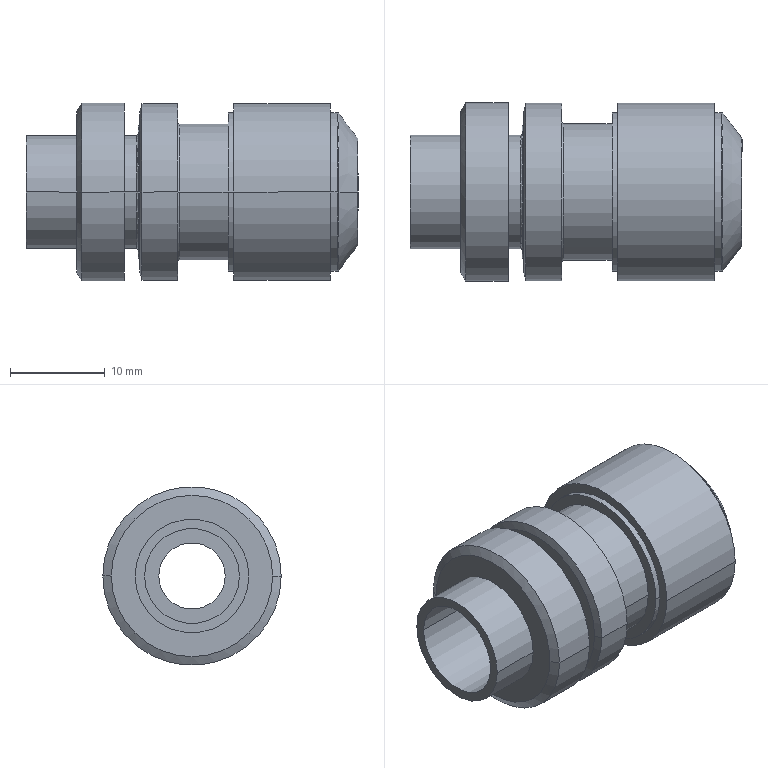Part | STEP file | AG12-6.5 | 1 solid | 47 faces | box 35 x 18.8 x 18.8 mm | volume 5027 mm3 | cylinder 22 | plane 11 | torus 8 | cone 6 | commonest cylinder face diameters 12 x4 16.7 x4 7 x2 10 x2 14 x2 14.4 x2
STEP:
#1=CARTESIAN_POINT('',(35.,3.5,0.));
#2=VERTEX_POINT('',#1);
#3=CARTESIAN_POINT('',(35.,-3.5,0.));
#4=VERTEX_POINT('',#3);
#5=CARTESIAN_POINT('',(35.,0.,0.));
#6=DIRECTION('',(-1.,0.,0.));
#7=DIRECTION('',(0.,1.,0.));
#8=AXIS2_PLACEMENT_3D('',#5,#6,#7);
#9=CIRCLE('',#8,3.5);
#10=EDGE_CURVE('',#2,#4,#9,.T.);
#11=ORIENTED_EDGE('',*,*,#10,.F.);
#12=CARTESIAN_POINT('',(30.,3.5,0.));
#13=VERTEX_POINT('',#12);
#14=CARTESIAN_POINT('',(35.001,3.5,0.));
#15=DIRECTION('',(-1.,0.,0.));
#16=VECTOR('',#15,1000.);
#17=LINE('',#14,#16);
#18=EDGE_CURVE('',#2,#13,#17,.T.);
#19=ORIENTED_EDGE('',*,*,#18,.T.);
#20=CARTESIAN_POINT('',(30.,-3.5,0.));
#21=VERTEX_POINT('',#20);
#22=CARTESIAN_POINT('',(30.,0.,0.));
#23=DIRECTION('',(-1.,0.,0.));
#24=DIRECTION('',(0.,-1.,0.));
#25=AXIS2_PLACEMENT_3D('',#22,#23,#24);
#26=CIRCLE('',#25,3.5);
#27=EDGE_CURVE('',#13,#21,#26,.T.);
#28=ORIENTED_EDGE('',*,*,#27,.T.);
#29=CARTESIAN_POINT('',(35.001,-3.5,0.));
#30=DIRECTION('',(-1.,0.,0.));
#31=VECTOR('',#30,1000.);
#32=LINE('',#29,#31);
#33=EDGE_CURVE('',#4,#21,#32,.T.);
#34=ORIENTED_EDGE('',*,*,#33,.F.);
#35=EDGE_LOOP('',(#11,#19,#28,#34));
#36=FACE_OUTER_BOUND('',#35,.T.);
#37=CARTESIAN_POINT('',(35.001,0.,0.));
#38=DIRECTION('',(-1.,0.,0.));
#39=DIRECTION('',(0.,-1.,0.));
#40=AXIS2_PLACEMENT_3D('',#37,#38,#39);
#41=CYLINDRICAL_SURFACE('',#40,3.5);
#42=ADVANCED_FACE('',(#36),#41,.F.);
#43=CARTESIAN_POINT('',(30.,5.,0.));
#44=VERTEX_POINT('',#43);
#45=CARTESIAN_POINT('',(30.,-5.,0.));
#46=VERTEX_POINT('',#45);
#47=CARTESIAN_POINT('',(30.,0.,0.));
#48=DIRECTION('',(-1.,0.,0.));
#49=DIRECTION('',(0.,-1.,0.));
#50=AXIS2_PLACEMENT_3D('',#47,#48,#49);
#51=CIRCLE('',#50,5.);
#52=EDGE_CURVE('',#44,#46,#51,.T.);
#53=ORIENTED_EDGE('',*,*,#52,.F.);
#54=CARTESIAN_POINT('',(0.,5.,0.));
#55=VERTEX_POINT('',#54);
#56=CARTESIAN_POINT('',(30.,5.,0.));
#57=DIRECTION('',(-1.,0.,0.));
#58=VECTOR('',#57,1000.);
#59=LINE('',#56,#58);
#60=EDGE_CURVE('',#44,#55,#59,.T.);
#61=ORIENTED_EDGE('',*,*,#60,.T.);
#62=CARTESIAN_POINT('',(0.,-5.,0.));
#63=VERTEX_POINT('',#62);
#64=CARTESIAN_POINT('',(0.,0.,0.));
#65=DIRECTION('',(-1.,0.,0.));
#66=DIRECTION('',(0.,-1.,0.));
#67=AXIS2_PLACEMENT_3D('',#64,#65,#66);
#68=CIRCLE('',#67,5.);
#69=EDGE_CURVE('',#55,#63,#68,.T.);
#70=ORIENTED_EDGE('',*,*,#69,.T.);
#71=CARTESIAN_POINT('',(30.,-5.,0.));
#72=DIRECTION('',(-1.,0.,0.));
#73=VECTOR('',#72,1000.);
#74=LINE('',#71,#73);
#75=EDGE_CURVE('',#46,#63,#74,.T.);
#76=ORIENTED_EDGE('',*,*,#75,.F.);
#77=EDGE_LOOP('',(#53,#61,#70,#76));
#78=FACE_OUTER_BOUND('',#77,.T.);
#79=CARTESIAN_POINT('',(30.,0.,0.));
#80=DIRECTION('',(-1.,0.,0.));
#81=DIRECTION('',(0.,-1.,0.));
#82=AXIS2_PLACEMENT_3D('',#79,#80,#81);
#83=CYLINDRICAL_SURFACE('',#82,5.);
#84=ADVANCED_FACE('',(#78),#83,.F.);
#85=CARTESIAN_POINT('',(12.,-7.,0.));
#86=VERTEX_POINT('',#85);
#87=CARTESIAN_POINT('',(12.,7.,0.));
#88=VERTEX_POINT('',#87);
#89=CARTESIAN_POINT('',(12.,0.,0.));
#90=DIRECTION('',(-1.,0.,0.));
#91=DIRECTION('',(0.,-1.,0.));
#92=AXIS2_PLACEMENT_3D('',#89,#90,#91);
#93=CIRCLE('',#92,7.);
#94=EDGE_CURVE('',#86,#88,#93,.T.);
#95=ORIENTED_EDGE('',*,*,#94,.T.);
#96=CARTESIAN_POINT('',(11.85,7.,0.));
#97=VERTEX_POINT('',#96);
#98=CARTESIAN_POINT('',(0.,7.,0.));
#99=DIRECTION('',(-1.,0.,0.));
#100=VECTOR('',#99,1000.);
#101=LINE('',#98,#100);
#102=EDGE_CURVE('',#88,#97,#101,.T.);
#103=ORIENTED_EDGE('',*,*,#102,.T.);
#104=CARTESIAN_POINT('',(11.85,-7.,0.));
#105=VERTEX_POINT('',#104);
#106=CARTESIAN_POINT('',(11.85,0.,0.));
#107=DIRECTION('',(-1.,0.,0.));
#108=DIRECTION('',(0.,-1.,0.));
#109=AXIS2_PLACEMENT_3D('',#106,#107,#108);
#110=CIRCLE('',#109,7.);
#111=EDGE_CURVE('',#105,#97,#110,.T.);
#112=ORIENTED_EDGE('',*,*,#111,.F.);
#113=CARTESIAN_POINT('',(0.,-7.,0.));
#114=DIRECTION('',(-1.,0.,0.));
#115=VECTOR('',#114,1000.);
#116=LINE('',#113,#115);
#117=EDGE_CURVE('',#86,#105,#116,.T.);
#118=ORIENTED_EDGE('',*,*,#117,.F.);
#119=EDGE_LOOP('',(#95,#103,#112,#118));
#120=FACE_OUTER_BOUND('',#119,.T.);
#121=CARTESIAN_POINT('',(0.,0.,0.));
#122=DIRECTION('',(-1.,0.,0.));
#123=DIRECTION('',(0.,-1.,0.));
#124=AXIS2_PLACEMENT_3D('',#121,#122,#123);
#125=CYLINDRICAL_SURFACE('',#124,7.);
#126=ADVANCED_FACE('',(#120),#125,.T.);
#127=CARTESIAN_POINT('',(12.,-8.5,0.));
#128=VERTEX_POINT('',#127);
#129=CARTESIAN_POINT('',(12.,8.5,0.));
#130=VERTEX_POINT('',#129);
#131=CARTESIAN_POINT('',(12.,0.,0.));
#132=DIRECTION('',(-1.,0.,0.));
#133=DIRECTION('',(0.,-1.,0.));
#134=AXIS2_PLACEMENT_3D('',#131,#132,#133);
#135=CIRCLE('',#134,8.5);
#136=EDGE_CURVE('',#128,#130,#135,.T.);
#137=ORIENTED_EDGE('',*,*,#136,.F.);
#138=CARTESIAN_POINT('',(12.228,-9.35,0.));
#139=VERTEX_POINT('',#138);
#140=CARTESIAN_POINT('',(12.,-8.5,0.));
#141=DIRECTION('',(0.2588,-0.9659,0.));
#142=VECTOR('',#141,1000.);
#143=LINE('',#140,#142);
#144=EDGE_CURVE('',#128,#139,#143,.T.);
#145=ORIENTED_EDGE('',*,*,#144,.T.);
#146=CARTESIAN_POINT('',(12.228,9.35,0.));
#147=VERTEX_POINT('',#146);
#148=CARTESIAN_POINT('',(12.228,0.,0.));
#149=DIRECTION('',(-1.,0.,0.));
#150=DIRECTION('',(0.,-1.,0.));
#151=AXIS2_PLACEMENT_3D('',#148,#149,#150);
#152=CIRCLE('',#151,9.35);
#153=EDGE_CURVE('',#139,#147,#152,.T.);
#154=ORIENTED_EDGE('',*,*,#153,.T.);
#155=CARTESIAN_POINT('',(12.,8.5,0.));
#156=DIRECTION('',(0.2588,0.9659,0.));
#157=VECTOR('',#156,1000.);
#158=LINE('',#155,#157);
#159=EDGE_CURVE('',#130,#147,#158,.T.);
#160=ORIENTED_EDGE('',*,*,#159,.F.);
#161=EDGE_LOOP('',(#137,#145,#154,#160));
#162=FACE_OUTER_BOUND('',#161,.T.);
#163=CARTESIAN_POINT('',(12.,0.,0.));
#164=DIRECTION('',(1.,0.,0.));
#165=DIRECTION('',(0.,1.,0.));
#166=AXIS2_PLACEMENT_3D('',#163,#164,#165);
#167=CONICAL_SURFACE('',#166,8.5,1.309);
#168=ADVANCED_FACE('',(#162),#167,.T.);
#169=CARTESIAN_POINT('',(16.,-9.35,0.));
#170=VERTEX_POINT('',#169);
#171=CARTESIAN_POINT('',(16.,9.35,0.));
#172=VERTEX_POINT('',#171);
#173=CARTESIAN_POINT('',(16.,0.,0.));
#174=DIRECTION('',(-1.,0.,0.));
#175=DIRECTION('',(0.,-1.,0.));
#176=AXIS2_PLACEMENT_3D('',#173,#174,#175);
#177=CIRCLE('',#176,9.35);
#178=EDGE_CURVE('',#170,#172,#177,.T.);
#179=ORIENTED_EDGE('',*,*,#178,.T.);
#180=CARTESIAN_POINT('',(0.,9.35,0.));
#181=DIRECTION('',(-1.,0.,0.));
#182=VECTOR('',#181,1000.);
#183=LINE('',#180,#182);
#184=EDGE_CURVE('',#172,#147,#183,.T.);
#185=ORIENTED_EDGE('',*,*,#184,.T.);
#186=ORIENTED_EDGE('',*,*,#153,.F.);
#187=CARTESIAN_POINT('',(0.,-9.35,0.));
#188=DIRECTION('',(-1.,0.,0.));
#189=VECTOR('',#188,1000.);
#190=LINE('',#187,#189);
#191=EDGE_CURVE('',#170,#139,#190,.T.);
#192=ORIENTED_EDGE('',*,*,#191,.F.);
#193=EDGE_LOOP('',(#179,#185,#186,#192));
#194=FACE_OUTER_BOUND('',#193,.T.);
#195=CARTESIAN_POINT('',(0.,0.,0.));
#196=DIRECTION('',(-1.,0.,0.));
#197=DIRECTION('',(0.,-1.,0.));
#198=AXIS2_PLACEMENT_3D('',#195,#196,#197);
#199=CYLINDRICAL_SURFACE('',#198,9.35);
#200=ADVANCED_FACE('',(#194),#199,.T.);
#201=CARTESIAN_POINT('',(16.,7.4,0.));
#202=VERTEX_POINT('',#201);
#203=CARTESIAN_POINT('',(16.,-7.4,0.));
#204=VERTEX_POINT('',#203);
#205=CARTESIAN_POINT('',(16.,0.,0.));
#206=DIRECTION('',(-1.,0.,0.));
#207=DIRECTION('',(0.,-1.,0.));
#208=AXIS2_PLACEMENT_3D('',#205,#206,#207);
#209=CIRCLE('',#208,7.4);
#210=EDGE_CURVE('',#202,#204,#209,.T.);
#211=ORIENTED_EDGE('',*,*,#210,.F.);
#212=CARTESIAN_POINT('',(16.2,7.2,0.));
#213=VERTEX_POINT('',#212);
#214=CARTESIAN_POINT('',(16.2,7.4,0.));
#215=DIRECTION('',(0.,0.,1.));
#216=DIRECTION('',(0.,-1.,0.));
#217=AXIS2_PLACEMENT_3D('',#214,#215,#216);
#218=CIRCLE('',#217,0.2);
#219=EDGE_CURVE('',#202,#213,#218,.T.);
#220=ORIENTED_EDGE('',*,*,#219,.T.);
#221=CARTESIAN_POINT('',(16.2,-7.2,0.));
#222=VERTEX_POINT('',#221);
#223=CARTESIAN_POINT('',(16.2,0.,0.));
#224=DIRECTION('',(-1.,0.,0.));
#225=DIRECTION('',(0.,-1.,0.));
#226=AXIS2_PLACEMENT_3D('',#223,#224,#225);
#227=CIRCLE('',#226,7.2);
#228=EDGE_CURVE('',#213,#222,#227,.T.);
#229=ORIENTED_EDGE('',*,*,#228,.T.);
#230=CARTESIAN_POINT('',(16.2,-7.4,0.));
#231=DIRECTION('',(0.,0.,-1.));
#232=DIRECTION('',(0.,1.,0.));
#233=AXIS2_PLACEMENT_3D('',#230,#231,#232);
#234=CIRCLE('',#233,0.2);
#235=EDGE_CURVE('',#204,#222,#234,.T.);
#236=ORIENTED_EDGE('',*,*,#235,.F.);
#237=EDGE_LOOP('',(#211,#220,#229,#236));
#238=FACE_OUTER_BOUND('',#237,.T.);
#239=CARTESIAN_POINT('',(16.2,0.,0.));
#240=DIRECTION('',(-1.,0.,0.));
#241=DIRECTION('',(0.,-1.,0.));
#242=AXIS2_PLACEMENT_3D('',#239,#240,#241);
#243=TOROIDAL_SURFACE('',#242,7.4,0.2);
#244=ADVANCED_FACE('',(#238),#243,.F.);
#245=CARTESIAN_POINT('',(21.3,-7.2,0.));
#246=VERTEX_POINT('',#245);
#247=CARTESIAN_POINT('',(21.3,7.2,0.));
#248=VERTEX_POINT('',#247);
#249=CARTESIAN_POINT('',(21.3,0.,0.));
#250=DIRECTION('',(-1.,0.,0.));
#251=DIRECTION('',(0.,-1.,0.));
#252=AXIS2_PLACEMENT_3D('',#249,#250,#251);
#253=CIRCLE('',#252,7.2);
#254=EDGE_CURVE('',#246,#248,#253,.T.);
#255=ORIENTED_EDGE('',*,*,#254,.T.);
#256=CARTESIAN_POINT('',(0.,7.2,0.));
#257=DIRECTION('',(-1.,0.,0.));
#258=VECTOR('',#257,1000.);
#259=LINE('',#256,#258);
#260=EDGE_CURVE('',#248,#213,#259,.T.);
#261=ORIENTED_EDGE('',*,*,#260,.T.);
#262=CARTESIAN_POINT('',(16.2,0.,0.));
#263=DIRECTION('',(-1.,0.,0.));
#264=DIRECTION('',(0.,-1.,0.));
#265=AXIS2_PLACEMENT_3D('',#262,#263,#264);
#266=CIRCLE('',#265,7.2);
#267=EDGE_CURVE('',#222,#213,#266,.T.);
#268=ORIENTED_EDGE('',*,*,#267,.F.);
#269=CARTESIAN_POINT('',(0.,-7.2,0.));
#270=DIRECTION('',(-1.,0.,0.));
#271=VECTOR('',#270,1000.);
#272=LINE('',#269,#271);
#273=EDGE_CURVE('',#246,#222,#272,.T.);
#274=ORIENTED_EDGE('',*,*,#273,.F.);
#275=EDGE_LOOP('',(#255,#261,#268,#274));
#276=FACE_OUTER_BOUND('',#275,.T.);
#277=CARTESIAN_POINT('',(0.,0.,0.));
#278=DIRECTION('',(-1.,0.,0.));
#279=DIRECTION('',(0.,-1.,0.));
#280=AXIS2_PLACEMENT_3D('',#277,#278,#279);
#281=CYLINDRICAL_SURFACE('',#280,7.2);
#282=ADVANCED_FACE('',(#276),#281,.T.);
#283=CARTESIAN_POINT('',(21.9,-8.35,0.));
#284=VERTEX_POINT('',#283);
#285=CARTESIAN_POINT('',(21.9,8.35,0.));
#286=VERTEX_POINT('',#285);
#287=CARTESIAN_POINT('',(21.9,0.,0.));
#288=DIRECTION('',(-1.,0.,0.));
#289=DIRECTION('',(0.,-1.,0.));
#290=AXIS2_PLACEMENT_3D('',#287,#288,#289);
#291=CIRCLE('',#290,8.35);
#292=EDGE_CURVE('',#284,#286,#291,.T.);
#293=ORIENTED_EDGE('',*,*,#292,.T.);
#294=CARTESIAN_POINT('',(21.3,8.35,0.));
#295=VERTEX_POINT('',#294);
#296=CARTESIAN_POINT('',(0.,8.35,0.));
#297=DIRECTION('',(-1.,0.,0.));
#298=VECTOR('',#297,1000.);
#299=LINE('',#296,#298);
#300=EDGE_CURVE('',#286,#295,#299,.T.);
#301=ORIENTED_EDGE('',*,*,#300,.T.);
#302=CARTESIAN_POINT('',(21.3,-8.35,0.));
#303=VERTEX_POINT('',#302);
#304=CARTESIAN_POINT('',(21.3,0.,0.));
#305=DIRECTION('',(-1.,0.,0.));
#306=DIRECTION('',(0.,-1.,0.));
#307=AXIS2_PLACEMENT_3D('',#304,#305,#306);
#308=CIRCLE('',#307,8.35);
#309=EDGE_CURVE('',#303,#295,#308,.T.);
#310=ORIENTED_EDGE('',*,*,#309,.F.);
#311=CARTESIAN_POINT('',(0.,-8.35,0.));
#312=DIRECTION('',(-1.,0.,0.));
#313=VECTOR('',#312,1000.);
#314=LINE('',#311,#313);
#315=EDGE_CURVE('',#284,#303,#314,.T.);
#316=ORIENTED_EDGE('',*,*,#315,.F.);
#317=EDGE_LOOP('',(#293,#301,#310,#316));
#318=FACE_OUTER_BOUND('',#317,.T.);
#319=CARTESIAN_POINT('',(0.,0.,0.));
#320=DIRECTION('',(-1.,0.,0.));
#321=DIRECTION('',(0.,-1.,0.));
#322=AXIS2_PLACEMENT_3D('',#319,#320,#321);
#323=CYLINDRICAL_SURFACE('',#322,8.35);
#324=ADVANCED_FACE('',(#318),#323,.T.);
#325=CARTESIAN_POINT('',(32.1,-9.365,0.));
#326=VERTEX_POINT('',#325);
#327=CARTESIAN_POINT('',(32.1,9.365,0.));
#328=VERTEX_POINT('',#327);
#329=CARTESIAN_POINT('',(32.1,0.,0.));
#330=DIRECTION('',(-1.,0.,0.));
#331=DIRECTION('',(0.,-1.,0.));
#332=AXIS2_PLACEMENT_3D('',#329,#330,#331);
#333=CIRCLE('',#332,9.365);
#334=EDGE_CURVE('',#326,#328,#333,.T.);
#335=ORIENTED_EDGE('',*,*,#334,.T.);
#336=CARTESIAN_POINT('',(21.9,9.365,0.));
#337=VERTEX_POINT('',#336);
#338=CARTESIAN_POINT('',(0.,9.365,0.));
#339=DIRECTION('',(-1.,0.,0.));
#340=VECTOR('',#339,1000.);
#341=LINE('',#338,#340);
#342=EDGE_CURVE('',#328,#337,#341,.T.);
#343=ORIENTED_EDGE('',*,*,#342,.T.);
#344=CARTESIAN_POINT('',(21.9,-9.365,0.));
#345=VERTEX_POINT('',#344);
#346=CARTESIAN_POINT('',(21.9,0.,0.));
#347=DIRECTION('',(-1.,0.,0.));
#348=DIRECTION('',(0.,-1.,0.));
#349=AXIS2_PLACEMENT_3D('',#346,#347,#348);
#350=CIRCLE('',#349,9.365);
#351=EDGE_CURVE('',#345,#337,#350,.T.);
#352=ORIENTED_EDGE('',*,*,#351,.F.);
#353=CARTESIAN_POINT('',(0.,-9.365,0.));
#354=DIRECTION('',(-1.,0.,0.));
#355=VECTOR('',#354,1000.);
#356=LINE('',#353,#355);
#357=EDGE_CURVE('',#326,#345,#356,.T.);
#358=ORIENTED_EDGE('',*,*,#357,.F.);
#359=EDGE_LOOP('',(#335,#343,#352,#358));
#360=FACE_OUTER_BOUND('',#359,.T.);
#361=CARTESIAN_POINT('',(0.,0.,0.));
#362=DIRECTION('',(-1.,0.,0.));
#363=DIRECTION('',(0.,-1.,0.));
#364=AXIS2_PLACEMENT_3D('',#361,#362,#363);
#365=CYLINDRICAL_SURFACE('',#364,9.365);
#366=ADVANCED_FACE('',(#360),#365,.T.);
#367=CARTESIAN_POINT('',(32.837,-8.35,0.));
#368=VERTEX_POINT('',#367);
#369=CARTESIAN_POINT('',(32.837,8.35,0.));
#370=VERTEX_POINT('',#369);
#371=CARTESIAN_POINT('',(32.837,0.,0.));
#372=DIRECTION('',(-1.,0.,0.));
#373=DIRECTION('',(0.,-1.,0.));
#374=AXIS2_PLACEMENT_3D('',#371,#372,#373);
#375=CIRCLE('',#374,8.35);
#376=EDGE_CURVE('',#368,#370,#375,.T.);
#377=ORIENTED_EDGE('',*,*,#376,.T.);
#378=CARTESIAN_POINT('',(32.1,8.35,0.));
#379=VERTEX_POINT('',#378);
#380=CARTESIAN_POINT('',(0.,8.35,0.));
#381=DIRECTION('',(-1.,0.,0.));
#382=VECTOR('',#381,1000.);
#383=LINE('',#380,#382);
#384=EDGE_CURVE('',#370,#379,#383,.T.);
#385=ORIENTED_EDGE('',*,*,#384,.T.);
#386=CARTESIAN_POINT('',(32.1,-8.35,0.));
#387=VERTEX_POINT('',#386);
#388=CARTESIAN_POINT('',(32.1,0.,0.));
#389=DIRECTION('',(-1.,0.,0.));
#390=DIRECTION('',(0.,-1.,0.));
#391=AXIS2_PLACEMENT_3D('',#388,#389,#390);
#392=CIRCLE('',#391,8.35);
#393=EDGE_CURVE('',#387,#379,#392,.T.);
#394=ORIENTED_EDGE('',*,*,#393,.F.);
#395=CARTESIAN_POINT('',(0.,-8.35,0.));
#396=DIRECTION('',(-1.,0.,0.));
#397=VECTOR('',#396,1000.);
#398=LINE('',#395,#397);
#399=EDGE_CURVE('',#368,#387,#398,.T.);
#400=ORIENTED_EDGE('',*,*,#399,.F.);
#401=EDGE_LOOP('',(#377,#385,#394,#400));
#402=FACE_OUTER_BOUND('',#401,.T.);
#403=CARTESIAN_POINT('',(0.,0.,0.));
#404=DIRECTION('',(-1.,0.,0.));
#405=DIRECTION('',(0.,-1.,0.));
#406=AXIS2_PLACEMENT_3D('',#403,#404,#405);
#407=CYLINDRICAL_SURFACE('',#406,8.35);
#408=ADVANCED_FACE('',(#402),#407,.T.);
#409=CARTESIAN_POINT('',(32.996,-8.271,0.));
#410=VERTEX_POINT('',#409);
#411=CARTESIAN_POINT('',(32.996,8.271,0.));
#412=VERTEX_POINT('',#411);
#413=CARTESIAN_POINT('',(32.996,0.,0.));
#414=DIRECTION('',(-1.,0.,0.));
#415=DIRECTION('',(0.,-1.,0.));
#416=AXIS2_PLACEMENT_3D('',#413,#414,#415);
#417=CIRCLE('',#416,8.271);
#418=EDGE_CURVE('',#410,#412,#417,.T.);
#419=ORIENTED_EDGE('',*,*,#418,.T.);
#420=CARTESIAN_POINT('',(32.837,8.15,0.));
#421=DIRECTION('',(0.,0.,1.));
#422=DIRECTION('',(0.,-1.,0.));
#423=AXIS2_PLACEMENT_3D('',#420,#421,#422);
#424=CIRCLE('',#423,0.2);
#425=EDGE_CURVE('',#412,#370,#424,.T.);
#426=ORIENTED_EDGE('',*,*,#425,.T.);
#427=ORIENTED_EDGE('',*,*,#376,.F.);
#428=CARTESIAN_POINT('',(32.837,-8.15,0.));
#429=DIRECTION('',(0.,0.,-1.));
#430=DIRECTION('',(0.,1.,0.));
#431=AXIS2_PLACEMENT_3D('',#428,#429,#430);
#432=CIRCLE('',#431,0.2);
#433=EDGE_CURVE('',#410,#368,#432,.T.);
#434=ORIENTED_EDGE('',*,*,#433,.F.);
#435=EDGE_LOOP('',(#419,#426,#427,#434));
#436=FACE_OUTER_BOUND('',#435,.T.);
#437=CARTESIAN_POINT('',(32.837,0.,0.));
#438=DIRECTION('',(-1.,0.,0.));
#439=DIRECTION('',(0.,-1.,0.));
#440=AXIS2_PLACEMENT_3D('',#437,#438,#439);
#441=TOROIDAL_SURFACE('',#440,8.15,0.2);
#442=ADVANCED_FACE('',(#436),#441,.T.);
#443=CARTESIAN_POINT('',(34.959,-5.704,0.));
#444=VERTEX_POINT('',#443);
#445=CARTESIAN_POINT('',(34.959,5.704,0.));
#446=VERTEX_POINT('',#445);
#447=CARTESIAN_POINT('',(34.959,0.,0.));
#448=DIRECTION('',(-1.,0.,0.));
#449=DIRECTION('',(0.,-1.,0.));
#450=AXIS2_PLACEMENT_3D('',#447,#448,#449);
#451=CIRCLE('',#450,5.704);
#452=EDGE_CURVE('',#444,#446,#451,.T.);
#453=ORIENTED_EDGE('',*,*,#452,.T.);
#454=CARTESIAN_POINT('',(34.959,5.704,0.));
#455=DIRECTION('',(-0.6074,0.7944,0.));
#456=VECTOR('',#455,1000.);
#457=LINE('',#454,#456);
#458=EDGE_CURVE('',#446,#412,#457,.T.);
#459=ORIENTED_EDGE('',*,*,#458,.T.);
#460=ORIENTED_EDGE('',*,*,#418,.F.);
#461=CARTESIAN_POINT('',(34.959,-5.704,0.));
#462=DIRECTION('',(-0.6074,-0.7944,0.));
#463=VECTOR('',#462,1000.);
#464=LINE('',#461,#463);
#465=EDGE_CURVE('',#444,#410,#464,.T.);
#466=ORIENTED_EDGE('',*,*,#465,.F.);
#467=EDGE_LOOP('',(#453,#459,#460,#466));
#468=FACE_OUTER_BOUND('',#467,.T.);
#469=CARTESIAN_POINT('',(34.959,0.,0.));
#470=DIRECTION('',(-1.,0.,0.));
#471=DIRECTION('',(0.,-1.,0.));
#472=AXIS2_PLACEMENT_3D('',#469,#470,#471);
#473=CONICAL_SURFACE('',#472,5.704,0.918);
#474=ADVANCED_FACE('',(#468),#473,.T.);
#475=CARTESIAN_POINT('',(35.,-5.582,0.));
#476=VERTEX_POINT('',#475);
#477=CARTESIAN_POINT('',(35.,5.582,0.));
#478=VERTEX_POINT('',#477);
#479=CARTESIAN_POINT('',(35.,0.,0.));
#480=DIRECTION('',(-1.,0.,0.));
#481=DIRECTION('',(0.,-1.,0.));
#482=AXIS2_PLACEMENT_3D('',#479,#480,#481);
#483=CIRCLE('',#482,5.582);
#484=EDGE_CURVE('',#476,#478,#483,.T.);
#485=ORIENTED_EDGE('',*,*,#484,.T.);
#486=CARTESIAN_POINT('',(34.8,5.582,0.));
#487=DIRECTION('',(0.,0.,1.));
#488=DIRECTION('',(0.,-1.,0.));
#489=AXIS2_PLACEMENT_3D('',#486,#487,#488);
#490=CIRCLE('',#489,0.2);
#491=EDGE_CURVE('',#478,#446,#490,.T.);
#492=ORIENTED_EDGE('',*,*,#491,.T.);
#493=ORIENTED_EDGE('',*,*,#452,.F.);
#494=CARTESIAN_POINT('',(34.8,-5.582,0.));
#495=DIRECTION('',(0.,0.,-1.));
#496=DIRECTION('',(0.,1.,0.));
#497=AXIS2_PLACEMENT_3D('',#494,#495,#496);
#498=CIRCLE('',#497,0.2);
#499=EDGE_CURVE('',#476,#444,#498,.T.);
#500=ORIENTED_EDGE('',*,*,#499,.F.);
#501=EDGE_LOOP('',(#485,#492,#493,#500));
#502=FACE_OUTER_BOUND('',#501,.T.);
#503=CARTESIAN_POINT('',(34.8,0.,0.));
#504=DIRECTION('',(-1.,0.,0.));
#505=DIRECTION('',(0.,-1.,0.));
#506=AXIS2_PLACEMENT_3D('',#503,#504,#505);
#507=TOROIDAL_SURFACE('',#506,5.582,0.2);
#508=ADVANCED_FACE('',(#502),#507,.T.);
#509=CARTESIAN_POINT('',(5.35,-6.,0.));
#510=VERTEX_POINT('',#509);
#511=CARTESIAN_POINT('',(5.35,6.,0.));
#512=VERTEX_POINT('',#511);
#513=CARTESIAN_POINT('',(5.35,0.,0.));
#514=DIRECTION('',(-1.,0.,0.));
#515=DIRECTION('',(0.,-1.,0.));
#516=AXIS2_PLACEMENT_3D('',#513,#514,#515);
#517=CIRCLE('',#516,6.);
#518=EDGE_CURVE('',#510,#512,#517,.T.);
#519=ORIENTED_EDGE('',*,*,#518,.T.);
#520=CARTESIAN_POINT('',(0.,6.,0.));
#521=VERTEX_POINT('',#520);
#522=CARTESIAN_POINT('',(0.,6.,0.));
#523=DIRECTION('',(-1.,0.,0.));
#524=VECTOR('',#523,1000.);
#525=LINE('',#522,#524);
#526=EDGE_CURVE('',#512,#521,#525,.T.);
#527=ORIENTED_EDGE('',*,*,#526,.T.);
#528=CARTESIAN_POINT('',(0.,-6.,0.));
#529=VERTEX_POINT('',#528);
#530=CARTESIAN_POINT('',(0.,0.,0.));
#531=DIRECTION('',(-1.,0.,0.));
#532=DIRECTION('',(0.,-1.,0.));
#533=AXIS2_PLACEMENT_3D('',#530,#531,#532);
#534=CIRCLE('',#533,6.);
#535=EDGE_CURVE('',#529,#521,#534,.T.);
#536=ORIENTED_EDGE('',*,*,#535,.F.);
#537=CARTESIAN_POINT('',(0.,-6.,0.));
#538=DIRECTION('',(-1.,0.,0.));
#539=VECTOR('',#538,1000.);
#540=LINE('',#537,#539);
#541=EDGE_CURVE('',#510,#529,#540,.T.);
#542=ORIENTED_EDGE('',*,*,#541,.F.);
#543=EDGE_LOOP('',(#519,#527,#536,#542));
#544=FACE_OUTER_BOUND('',#543,.T.);
#545=CARTESIAN_POINT('',(0.,0.,0.));
#546=DIRECTION('',(-1.,0.,0.));
#547=DIRECTION('',(0.,-1.,0.));
#548=AXIS2_PLACEMENT_3D('',#545,#546,#547);
#549=CYLINDRICAL_SURFACE('',#548,6.);
#550=ADVANCED_FACE('',(#544),#549,.T.);
#551=CARTESIAN_POINT('',(5.35,-8.5,0.));
#552=VERTEX_POINT('',#551);
#553=CARTESIAN_POINT('',(5.35,8.5,0.));
#554=VERTEX_POINT('',#553);
#555=CARTESIAN_POINT('',(5.35,0.,0.));
#556=DIRECTION('',(-1.,0.,0.));
#557=DIRECTION('',(0.,-1.,0.));
#558=AXIS2_PLACEMENT_3D('',#555,#556,#557);
#559=CIRCLE('',#558,8.5);
#560=EDGE_CURVE('',#552,#554,#559,.T.);
#561=ORIENTED_EDGE('',*,*,#560,.F.);
#562=CARTESIAN_POINT('',(5.87,-9.4,0.));
#563=VERTEX_POINT('',#562);
#564=CARTESIAN_POINT('',(5.35,-8.5,0.));
#565=DIRECTION('',(0.5,-0.866,0.));
#566=VECTOR('',#565,1000.);
#567=LINE('',#564,#566);
#568=EDGE_CURVE('',#552,#563,#567,.T.);
#569=ORIENTED_EDGE('',*,*,#568,.T.);
#570=CARTESIAN_POINT('',(5.87,9.4,0.));
#571=VERTEX_POINT('',#570);
#572=CARTESIAN_POINT('',(5.87,0.,0.));
#573=DIRECTION('',(-1.,0.,0.));
#574=DIRECTION('',(0.,-1.,0.));
#575=AXIS2_PLACEMENT_3D('',#572,#573,#574);
#576=CIRCLE('',#575,9.4);
#577=EDGE_CURVE('',#563,#571,#576,.T.);
#578=ORIENTED_EDGE('',*,*,#577,.T.);
#579=CARTESIAN_POINT('',(5.35,8.5,0.));
#580=DIRECTION('',(0.5,0.866,0.));
#581=VECTOR('',#580,1000.);
#582=LINE('',#579,#581);
#583=EDGE_CURVE('',#554,#571,#582,.T.);
#584=ORIENTED_EDGE('',*,*,#583,.F.);
#585=EDGE_LOOP('',(#561,#569,#578,#584));
#586=FACE_OUTER_BOUND('',#585,.T.);
#587=CARTESIAN_POINT('',(5.35,0.,0.));
#588=DIRECTION('',(1.,0.,0.));
#589=DIRECTION('',(0.,1.,0.));
#590=AXIS2_PLACEMENT_3D('',#587,#588,#589);
#591=CONICAL_SURFACE('',#590,8.5,1.047);
#592=ADVANCED_FACE('',(#586),#591,.T.);
#593=CARTESIAN_POINT('',(10.35,-9.4,0.));
#594=VERTEX_POINT('',#593);
#595=CARTESIAN_POINT('',(10.35,9.4,0.));
#596=VERTEX_POINT('',#595);
#597=CARTESIAN_POINT('',(10.35,0.,0.));
#598=DIRECTION('',(-1.,0.,0.));
#599=DIRECTION('',(0.,-1.,0.));
#600=AXIS2_PLACEMENT_3D('',#597,#598,#599);
#601=CIRCLE('',#600,9.4);
#602=EDGE_CURVE('',#594,#596,#601,.T.);
#603=ORIENTED_EDGE('',*,*,#602,.T.);
#604=CARTESIAN_POINT('',(0.,9.4,0.));
#605=DIRECTION('',(-1.,0.,0.));
#606=VECTOR('',#605,1000.);
#607=LINE('',#604,#606);
#608=EDGE_CURVE('',#596,#571,#607,.T.);
#609=ORIENTED_EDGE('',*,*,#608,.T.);
#610=ORIENTED_EDGE('',*,*,#577,.F.);
#611=CARTESIAN_POINT('',(0.,-9.4,0.));
#612=DIRECTION('',(-1.,0.,0.));
#613=VECTOR('',#612,1000.);
#614=LINE('',#611,#613);
#615=EDGE_CURVE('',#594,#563,#614,.T.);
#616=ORIENTED_EDGE('',*,*,#615,.F.);
#617=EDGE_LOOP('',(#603,#609,#610,#616));
#618=FACE_OUTER_BOUND('',#617,.T.);
#619=CARTESIAN_POINT('',(0.,0.,0.));
#620=DIRECTION('',(-1.,0.,0.));
#621=DIRECTION('',(0.,-1.,0.));
#622=AXIS2_PLACEMENT_3D('',#619,#620,#621);
#623=CYLINDRICAL_SURFACE('',#622,9.4);
#624=ADVANCED_FACE('',(#618),#623,.T.);
#625=CARTESIAN_POINT('',(11.65,-6.,0.));
#626=VERTEX_POINT('',#625);
#627=CARTESIAN_POINT('',(11.65,6.,0.));
#628=VERTEX_POINT('',#627);
#629=CARTESIAN_POINT('',(11.65,0.,0.));
#630=DIRECTION('',(-1.,0.,0.));
#631=DIRECTION('',(0.,-1.,0.));
#632=AXIS2_PLACEMENT_3D('',#629,#630,#631);
#633=CIRCLE('',#632,6.);
#634=EDGE_CURVE('',#626,#628,#633,.T.);
#635=ORIENTED_EDGE('',*,*,#634,.T.);
#636=CARTESIAN_POINT('',(10.35,6.,0.));
#637=VERTEX_POINT('',#636);
#638=CARTESIAN_POINT('',(0.,6.,0.));
#639=DIRECTION('',(-1.,0.,0.));
#640=VECTOR('',#639,1000.);
#641=LINE('',#638,#640);
#642=EDGE_CURVE('',#628,#637,#641,.T.);
#643=ORIENTED_EDGE('',*,*,#642,.T.);
#644=CARTESIAN_POINT('',(10.35,-6.,0.));
#645=VERTEX_POINT('',#644);
#646=CARTESIAN_POINT('',(10.35,0.,0.));
#647=DIRECTION('',(-1.,0.,0.));
#648=DIRECTION('',(0.,-1.,0.));
#649=AXIS2_PLACEMENT_3D('',#646,#647,#648);
#650=CIRCLE('',#649,6.);
#651=EDGE_CURVE('',#645,#637,#650,.T.);
#652=ORIENTED_EDGE('',*,*,#651,.F.);
#653=CARTESIAN_POINT('',(0.,-6.,0.));
#654=DIRECTION('',(-1.,0.,0.));
#655=VECTOR('',#654,1000.);
#656=LINE('',#653,#655);
#657=EDGE_CURVE('',#626,#645,#656,.T.);
#658=ORIENTED_EDGE('',*,*,#657,.F.);
#659=EDGE_LOOP('',(#635,#643,#652,#658));
#660=FACE_OUTER_BOUND('',#659,.T.);
#661=CARTESIAN_POINT('',(0.,0.,0.));
#662=DIRECTION('',(-1.,0.,0.));
#663=DIRECTION('',(0.,-1.,0.));
#664=AXIS2_PLACEMENT_3D('',#661,#662,#663);
#665=CYLINDRICAL_SURFACE('',#664,6.);
#666=ADVANCED_FACE('',(#660),#665,.T.);
#667=CARTESIAN_POINT('',(11.65,0.,0.));
#668=DIRECTION('',(-1.,0.,0.));
#669=DIRECTION('',(0.,-1.,0.));
#670=AXIS2_PLACEMENT_3D('',#667,#668,#669);
#671=CIRCLE('',#670,6.);
#672=EDGE_CURVE('',#628,#626,#671,.T.);
#673=ORIENTED_EDGE('',*,*,#672,.F.);
#674=CARTESIAN_POINT('',(11.85,6.2,0.));
#675=VERTEX_POINT('',#674);
#676=CARTESIAN_POINT('',(11.65,6.2,0.));
#677=DIRECTION('',(0.,0.,1.));
#678=DIRECTION('',(0.,-1.,0.));
#679=AXIS2_PLACEMENT_3D('',#676,#677,#678);
#680=CIRCLE('',#679,0.2);
#681=EDGE_CURVE('',#628,#675,#680,.T.);
#682=ORIENTED_EDGE('',*,*,#681,.T.);
#683=CARTESIAN_POINT('',(11.85,-6.2,0.));
#684=VERTEX_POINT('',#683);
#685=CARTESIAN_POINT('',(11.85,0.,0.));
#686=DIRECTION('',(-1.,0.,0.));
#687=DIRECTION('',(0.,-1.,0.));
#688=AXIS2_PLACEMENT_3D('',#685,#686,#687);
#689=CIRCLE('',#688,6.2);
#690=EDGE_CURVE('',#675,#684,#689,.T.);
#691=ORIENTED_EDGE('',*,*,#690,.T.);
#692=CARTESIAN_POINT('',(11.65,-6.2,0.));
#693=DIRECTION('',(0.,0.,-1.));
#694=DIRECTION('',(0.,1.,0.));
#695=AXIS2_PLACEMENT_3D('',#692,#693,#694);
#696=CIRCLE('',#695,0.2);
#697=EDGE_CURVE('',#626,#684,#696,.T.);
#698=ORIENTED_EDGE('',*,*,#697,.F.);
#699=EDGE_LOOP('',(#673,#682,#691,#698));
#700=FACE_OUTER_BOUND('',#699,.T.);
#701=CARTESIAN_POINT('',(11.65,0.,0.));
#702=DIRECTION('',(-1.,0.,0.));
#703=DIRECTION('',(0.,-1.,0.));
#704=AXIS2_PLACEMENT_3D('',#701,#702,#703);
#705=TOROIDAL_SURFACE('',#704,6.2,0.2);
#706=ADVANCED_FACE('',(#700),#705,.F.);
#707=ORIENTED_EDGE('',*,*,#681,.F.);
#708=ORIENTED_EDGE('',*,*,#634,.F.);
#709=ORIENTED_EDGE('',*,*,#697,.T.);
#710=CARTESIAN_POINT('',(11.85,0.,0.));
#711=DIRECTION('',(-1.,0.,0.));
#712=DIRECTION('',(0.,-1.,0.));
#713=AXIS2_PLACEMENT_3D('',#710,#711,#712);
#714=CIRCLE('',#713,6.2);
#715=EDGE_CURVE('',#684,#675,#714,.T.);
#716=ORIENTED_EDGE('',*,*,#715,.T.);
#717=EDGE_LOOP('',(#707,#708,#709,#716));
#718=FACE_OUTER_BOUND('',#717,.T.);
#719=CARTESIAN_POINT('',(11.65,0.,0.));
#720=DIRECTION('',(-1.,0.,0.));
#721=DIRECTION('',(0.,-1.,0.));
#722=AXIS2_PLACEMENT_3D('',#719,#720,#721);
#723=TOROIDAL_SURFACE('',#722,6.2,0.2);
#724=ADVANCED_FACE('',(#718),#723,.F.);
#725=ORIENTED_EDGE('',*,*,#642,.F.);
#726=ORIENTED_EDGE('',*,*,#672,.T.);
#727=ORIENTED_EDGE('',*,*,#657,.T.);
#728=CARTESIAN_POINT('',(10.35,0.,0.));
#729=DIRECTION('',(-1.,0.,0.));
#730=DIRECTION('',(0.,-1.,0.));
#731=AXIS2_PLACEMENT_3D('',#728,#729,#730);
#732=CIRCLE('',#731,6.);
#733=EDGE_CURVE('',#637,#645,#732,.T.);
#734=ORIENTED_EDGE('',*,*,#733,.F.);
#735=EDGE_LOOP('',(#725,#726,#727,#734));
#736=FACE_OUTER_BOUND('',#735,.T.);
#737=CARTESIAN_POINT('',(0.,0.,0.));
#738=DIRECTION('',(-1.,0.,0.));
#739=DIRECTION('',(0.,-1.,0.));
#740=AXIS2_PLACEMENT_3D('',#737,#738,#739);
#741=CYLINDRICAL_SURFACE('',#740,6.);
#742=ADVANCED_FACE('',(#736),#741,.T.);
#743=ORIENTED_EDGE('',*,*,#651,.T.);
#744=ORIENTED_EDGE('',*,*,#733,.T.);
#745=EDGE_LOOP('',(#743,#744));
#746=FACE_BOUND('',#745,.T.);
#747=ORIENTED_EDGE('',*,*,#602,.F.);
#748=CARTESIAN_POINT('',(10.35,0.,0.));
#749=DIRECTION('',(-1.,0.,0.));
#750=DIRECTION('',(0.,-1.,0.));
#751=AXIS2_PLACEMENT_3D('',#748,#749,#750);
#752=CIRCLE('',#751,9.4);
#753=EDGE_CURVE('',#596,#594,#752,.T.);
#754=ORIENTED_EDGE('',*,*,#753,.F.);
#755=EDGE_LOOP('',(#747,#754));
#756=FACE_OUTER_BOUND('',#755,.T.);
#757=CARTESIAN_POINT('',(10.35,0.,0.));
#758=DIRECTION('',(1.,0.,0.));
#759=DIRECTION('',(0.,1.,0.));
#760=AXIS2_PLACEMENT_3D('',#757,#758,#759);
#761=PLANE('',#760);
#762=ADVANCED_FACE('',(#746,#756),#761,.T.);
#763=ORIENTED_EDGE('',*,*,#608,.F.);
#764=ORIENTED_EDGE('',*,*,#753,.T.);
#765=ORIENTED_EDGE('',*,*,#615,.T.);
#766=CARTESIAN_POINT('',(5.87,0.,0.));
#767=DIRECTION('',(-1.,0.,0.));
#768=DIRECTION('',(0.,-1.,0.));
#769=AXIS2_PLACEMENT_3D('',#766,#767,#768);
#770=CIRCLE('',#769,9.4);
#771=EDGE_CURVE('',#571,#563,#770,.T.);
#772=ORIENTED_EDGE('',*,*,#771,.F.);
#773=EDGE_LOOP('',(#763,#764,#765,#772));
#774=FACE_OUTER_BOUND('',#773,.T.);
#775=CARTESIAN_POINT('',(0.,0.,0.));
#776=DIRECTION('',(-1.,0.,0.));
#777=DIRECTION('',(0.,-1.,0.));
#778=AXIS2_PLACEMENT_3D('',#775,#776,#777);
#779=CYLINDRICAL_SURFACE('',#778,9.4);
#780=ADVANCED_FACE('',(#774),#779,.T.);
#781=ORIENTED_EDGE('',*,*,#568,.F.);
#782=CARTESIAN_POINT('',(5.35,0.,0.));
#783=DIRECTION('',(-1.,0.,0.));
#784=DIRECTION('',(0.,-1.,0.));
#785=AXIS2_PLACEMENT_3D('',#782,#783,#784);
#786=CIRCLE('',#785,8.5);
#787=EDGE_CURVE('',#554,#552,#786,.T.);
#788=ORIENTED_EDGE('',*,*,#787,.F.);
#789=ORIENTED_EDGE('',*,*,#583,.T.);
#790=ORIENTED_EDGE('',*,*,#771,.T.);
#791=EDGE_LOOP('',(#781,#788,#789,#790));
#792=FACE_OUTER_BOUND('',#791,.T.);
#793=CARTESIAN_POINT('',(5.35,0.,0.));
#794=DIRECTION('',(1.,0.,0.));
#795=DIRECTION('',(0.,1.,0.));
#796=AXIS2_PLACEMENT_3D('',#793,#794,#795);
#797=CONICAL_SURFACE('',#796,8.5,1.047);
#798=ADVANCED_FACE('',(#792),#797,.T.);
#799=ORIENTED_EDGE('',*,*,#518,.F.);
#800=CARTESIAN_POINT('',(5.35,0.,0.));
#801=DIRECTION('',(-1.,0.,0.));
#802=DIRECTION('',(0.,-1.,0.));
#803=AXIS2_PLACEMENT_3D('',#800,#801,#802);
#804=CIRCLE('',#803,6.);
#805=EDGE_CURVE('',#512,#510,#804,.T.);
#806=ORIENTED_EDGE('',*,*,#805,.F.);
#807=EDGE_LOOP('',(#799,#806));
#808=FACE_BOUND('',#807,.T.);
#809=ORIENTED_EDGE('',*,*,#787,.T.);
#810=ORIENTED_EDGE('',*,*,#560,.T.);
#811=EDGE_LOOP('',(#809,#810));
#812=FACE_OUTER_BOUND('',#811,.T.);
#813=CARTESIAN_POINT('',(5.35,0.,0.));
#814=DIRECTION('',(1.,0.,0.));
#815=DIRECTION('',(0.,1.,0.));
#816=AXIS2_PLACEMENT_3D('',#813,#814,#815);
#817=PLANE('',#816);
#818=ADVANCED_FACE('',(#808,#812),#817,.F.);
#819=ORIENTED_EDGE('',*,*,#526,.F.);
#820=ORIENTED_EDGE('',*,*,#805,.T.);
#821=ORIENTED_EDGE('',*,*,#541,.T.);
#822=CARTESIAN_POINT('',(0.,0.,0.));
#823=DIRECTION('',(-1.,0.,0.));
#824=DIRECTION('',(0.,-1.,0.));
#825=AXIS2_PLACEMENT_3D('',#822,#823,#824);
#826=CIRCLE('',#825,6.);
#827=EDGE_CURVE('',#521,#529,#826,.T.);
#828=ORIENTED_EDGE('',*,*,#827,.F.);
#829=EDGE_LOOP('',(#819,#820,#821,#828));
#830=FACE_OUTER_BOUND('',#829,.T.);
#831=CARTESIAN_POINT('',(0.,0.,0.));
#832=DIRECTION('',(-1.,0.,0.));
#833=DIRECTION('',(0.,-1.,0.));
#834=AXIS2_PLACEMENT_3D('',#831,#832,#833);
#835=CYLINDRICAL_SURFACE('',#834,6.);
#836=ADVANCED_FACE('',(#830),#835,.T.);
#837=CARTESIAN_POINT('',(0.,0.,0.));
#838=DIRECTION('',(-1.,0.,0.));
#839=DIRECTION('',(0.,-1.,0.));
#840=AXIS2_PLACEMENT_3D('',#837,#838,#839);
#841=CIRCLE('',#840,5.);
#842=EDGE_CURVE('',#63,#55,#841,.T.);
#843=ORIENTED_EDGE('',*,*,#842,.F.);
#844=ORIENTED_EDGE('',*,*,#69,.F.);
#845=EDGE_LOOP('',(#843,#844));
#846=FACE_BOUND('',#845,.T.);
#847=ORIENTED_EDGE('',*,*,#535,.T.);
#848=ORIENTED_EDGE('',*,*,#827,.T.);
#849=EDGE_LOOP('',(#847,#848));
#850=FACE_OUTER_BOUND('',#849,.T.);
#851=CARTESIAN_POINT('',(0.,0.,0.));
#852=DIRECTION('',(1.,0.,0.));
#853=DIRECTION('',(0.,1.,0.));
#854=AXIS2_PLACEMENT_3D('',#851,#852,#853);
#855=PLANE('',#854);
#856=ADVANCED_FACE('',(#846,#850),#855,.F.);
#857=CARTESIAN_POINT('',(35.,0.,0.));
#858=DIRECTION('',(-1.,0.,0.));
#859=DIRECTION('',(0.,1.,0.));
#860=AXIS2_PLACEMENT_3D('',#857,#858,#859);
#861=CIRCLE('',#860,3.5);
#862=EDGE_CURVE('',#4,#2,#861,.T.);
#863=ORIENTED_EDGE('',*,*,#862,.T.);
#864=ORIENTED_EDGE('',*,*,#10,.T.);
#865=EDGE_LOOP('',(#863,#864));
#866=FACE_BOUND('',#865,.T.);
#867=ORIENTED_EDGE('',*,*,#484,.F.);
#868=CARTESIAN_POINT('',(35.,0.,0.));
#869=DIRECTION('',(-1.,0.,0.));
#870=DIRECTION('',(0.,-1.,0.));
#871=AXIS2_PLACEMENT_3D('',#868,#869,#870);
#872=CIRCLE('',#871,5.582);
#873=EDGE_CURVE('',#478,#476,#872,.T.);
#874=ORIENTED_EDGE('',*,*,#873,.F.);
#875=EDGE_LOOP('',(#867,#874));
#876=FACE_OUTER_BOUND('',#875,.T.);
#877=CARTESIAN_POINT('',(35.,0.,0.));
#878=DIRECTION('',(1.,0.,0.));
#879=DIRECTION('',(0.,1.,0.));
#880=AXIS2_PLACEMENT_3D('',#877,#878,#879);
#881=PLANE('',#880);
#882=ADVANCED_FACE('',(#866,#876),#881,.T.);
#883=ORIENTED_EDGE('',*,*,#491,.F.);
#884=ORIENTED_EDGE('',*,*,#873,.T.);
#885=ORIENTED_EDGE('',*,*,#499,.T.);
#886=CARTESIAN_POINT('',(34.959,0.,0.));
#887=DIRECTION('',(-1.,0.,0.));
#888=DIRECTION('',(0.,-1.,0.));
#889=AXIS2_PLACEMENT_3D('',#886,#887,#888);
#890=CIRCLE('',#889,5.704);
#891=EDGE_CURVE('',#446,#444,#890,.T.);
#892=ORIENTED_EDGE('',*,*,#891,.F.);
#893=EDGE_LOOP('',(#883,#884,#885,#892));
#894=FACE_OUTER_BOUND('',#893,.T.);
#895=CARTESIAN_POINT('',(34.8,0.,0.));
#896=DIRECTION('',(-1.,0.,0.));
#897=DIRECTION('',(0.,-1.,0.));
#898=AXIS2_PLACEMENT_3D('',#895,#896,#897);
#899=TOROIDAL_SURFACE('',#898,5.582,0.2);
#900=ADVANCED_FACE('',(#894),#899,.T.);
#901=ORIENTED_EDGE('',*,*,#458,.F.);
#902=ORIENTED_EDGE('',*,*,#891,.T.);
#903=ORIENTED_EDGE('',*,*,#465,.T.);
#904=CARTESIAN_POINT('',(32.996,0.,0.));
#905=DIRECTION('',(-1.,0.,0.));
#906=DIRECTION('',(0.,-1.,0.));
#907=AXIS2_PLACEMENT_3D('',#904,#905,#906);
#908=CIRCLE('',#907,8.271);
#909=EDGE_CURVE('',#412,#410,#908,.T.);
#910=ORIENTED_EDGE('',*,*,#909,.F.);
#911=EDGE_LOOP('',(#901,#902,#903,#910));
#912=FACE_OUTER_BOUND('',#911,.T.);
#913=CARTESIAN_POINT('',(34.959,0.,0.));
#914=DIRECTION('',(-1.,0.,0.));
#915=DIRECTION('',(0.,-1.,0.));
#916=AXIS2_PLACEMENT_3D('',#913,#914,#915);
#917=CONICAL_SURFACE('',#916,5.704,0.918);
#918=ADVANCED_FACE('',(#912),#917,.T.);
#919=ORIENTED_EDGE('',*,*,#425,.F.);
#920=ORIENTED_EDGE('',*,*,#909,.T.);
#921=ORIENTED_EDGE('',*,*,#433,.T.);
#922=CARTESIAN_POINT('',(32.837,0.,0.));
#923=DIRECTION('',(-1.,0.,0.));
#924=DIRECTION('',(0.,-1.,0.));
#925=AXIS2_PLACEMENT_3D('',#922,#923,#924);
#926=CIRCLE('',#925,8.35);
#927=EDGE_CURVE('',#370,#368,#926,.T.);
#928=ORIENTED_EDGE('',*,*,#927,.F.);
#929=EDGE_LOOP('',(#919,#920,#921,#928));
#930=FACE_OUTER_BOUND('',#929,.T.);
#931=CARTESIAN_POINT('',(32.837,0.,0.));
#932=DIRECTION('',(-1.,0.,0.));
#933=DIRECTION('',(0.,-1.,0.));
#934=AXIS2_PLACEMENT_3D('',#931,#932,#933);
#935=TOROIDAL_SURFACE('',#934,8.15,0.2);
#936=ADVANCED_FACE('',(#930),#935,.T.);
#937=ORIENTED_EDGE('',*,*,#384,.F.);
#938=ORIENTED_EDGE('',*,*,#927,.T.);
#939=ORIENTED_EDGE('',*,*,#399,.T.);
#940=CARTESIAN_POINT('',(32.1,0.,0.));
#941=DIRECTION('',(-1.,0.,0.));
#942=DIRECTION('',(0.,-1.,0.));
#943=AXIS2_PLACEMENT_3D('',#940,#941,#942);
#944=CIRCLE('',#943,8.35);
#945=EDGE_CURVE('',#379,#387,#944,.T.);
#946=ORIENTED_EDGE('',*,*,#945,.F.);
#947=EDGE_LOOP('',(#937,#938,#939,#946));
#948=FACE_OUTER_BOUND('',#947,.T.);
#949=CARTESIAN_POINT('',(0.,0.,0.));
#950=DIRECTION('',(-1.,0.,0.));
#951=DIRECTION('',(0.,-1.,0.));
#952=AXIS2_PLACEMENT_3D('',#949,#950,#951);
#953=CYLINDRICAL_SURFACE('',#952,8.35);
#954=ADVANCED_FACE('',(#948),#953,.T.);
#955=ORIENTED_EDGE('',*,*,#393,.T.);
#956=ORIENTED_EDGE('',*,*,#945,.T.);
#957=EDGE_LOOP('',(#955,#956));
#958=FACE_BOUND('',#957,.T.);
#959=ORIENTED_EDGE('',*,*,#334,.F.);
#960=CARTESIAN_POINT('',(32.1,0.,0.));
#961=DIRECTION('',(-1.,0.,0.));
#962=DIRECTION('',(0.,-1.,0.));
#963=AXIS2_PLACEMENT_3D('',#960,#961,#962);
#964=CIRCLE('',#963,9.365);
#965=EDGE_CURVE('',#328,#326,#964,.T.);
#966=ORIENTED_EDGE('',*,*,#965,.F.);
#967=EDGE_LOOP('',(#959,#966));
#968=FACE_OUTER_BOUND('',#967,.T.);
#969=CARTESIAN_POINT('',(32.1,0.,0.));
#970=DIRECTION('',(1.,0.,0.));
#971=DIRECTION('',(0.,1.,0.));
#972=AXIS2_PLACEMENT_3D('',#969,#970,#971);
#973=PLANE('',#972);
#974=ADVANCED_FACE('',(#958,#968),#973,.T.);
#975=ORIENTED_EDGE('',*,*,#342,.F.);
#976=ORIENTED_EDGE('',*,*,#965,.T.);
#977=ORIENTED_EDGE('',*,*,#357,.T.);
#978=CARTESIAN_POINT('',(21.9,0.,0.));
#979=DIRECTION('',(-1.,0.,0.));
#980=DIRECTION('',(0.,-1.,0.));
#981=AXIS2_PLACEMENT_3D('',#978,#979,#980);
#982=CIRCLE('',#981,9.365);
#983=EDGE_CURVE('',#337,#345,#982,.T.);
#984=ORIENTED_EDGE('',*,*,#983,.F.);
#985=EDGE_LOOP('',(#975,#976,#977,#984));
#986=FACE_OUTER_BOUND('',#985,.T.);
#987=CARTESIAN_POINT('',(0.,0.,0.));
#988=DIRECTION('',(-1.,0.,0.));
#989=DIRECTION('',(0.,-1.,0.));
#990=AXIS2_PLACEMENT_3D('',#987,#988,#989);
#991=CYLINDRICAL_SURFACE('',#990,9.365);
#992=ADVANCED_FACE('',(#986),#991,.T.);
#993=ORIENTED_EDGE('',*,*,#292,.F.);
#994=CARTESIAN_POINT('',(21.9,0.,0.));
#995=DIRECTION('',(-1.,0.,0.));
#996=DIRECTION('',(0.,-1.,0.));
#997=AXIS2_PLACEMENT_3D('',#994,#995,#996);
#998=CIRCLE('',#997,8.35);
#999=EDGE_CURVE('',#286,#284,#998,.T.);
#1000=ORIENTED_EDGE('',*,*,#999,.F.);
#1001=EDGE_LOOP('',(#993,#1000));
#1002=FACE_BOUND('',#1001,.T.);
#1003=ORIENTED_EDGE('',*,*,#351,.T.);
#1004=ORIENTED_EDGE('',*,*,#983,.T.);
#1005=EDGE_LOOP('',(#1003,#1004));
#1006=FACE_OUTER_BOUND('',#1005,.T.);
#1007=CARTESIAN_POINT('',(21.9,0.,0.));
#1008=DIRECTION('',(1.,0.,0.));
#1009=DIRECTION('',(0.,1.,0.));
#1010=AXIS2_PLACEMENT_3D('',#1007,#1008,#1009);
#1011=PLANE('',#1010);
#1012=ADVANCED_FACE('',(#1002,#1006),#1011,.F.);
#1013=ORIENTED_EDGE('',*,*,#300,.F.);
#1014=ORIENTED_EDGE('',*,*,#999,.T.);
#1015=ORIENTED_EDGE('',*,*,#315,.T.);
#1016=CARTESIAN_POINT('',(21.3,0.,0.));
#1017=DIRECTION('',(-1.,0.,0.));
#1018=DIRECTION('',(0.,-1.,0.));
#1019=AXIS2_PLACEMENT_3D('',#1016,#1017,#1018);
#1020=CIRCLE('',#1019,8.35);
#1021=EDGE_CURVE('',#295,#303,#1020,.T.);
#1022=ORIENTED_EDGE('',*,*,#1021,.F.);
#1023=EDGE_LOOP('',(#1013,#1014,#1015,#1022));
#1024=FACE_OUTER_BOUND('',#1023,.T.);
#1025=CARTESIAN_POINT('',(0.,0.,0.));
#1026=DIRECTION('',(-1.,0.,0.));
#1027=DIRECTION('',(0.,-1.,0.));
#1028=AXIS2_PLACEMENT_3D('',#1025,#1026,#1027);
#1029=CYLINDRICAL_SURFACE('',#1028,8.35);
#1030=ADVANCED_FACE('',(#1024),#1029,.T.);
#1031=ORIENTED_EDGE('',*,*,#254,.F.);
#1032=CARTESIAN_POINT('',(21.3,0.,0.));
#1033=DIRECTION('',(-1.,0.,0.));
#1034=DIRECTION('',(0.,-1.,0.));
#1035=AXIS2_PLACEMENT_3D('',#1032,#1033,#1034);
#1036=CIRCLE('',#1035,7.2);
#1037=EDGE_CURVE('',#248,#246,#1036,.T.);
#1038=ORIENTED_EDGE('',*,*,#1037,.F.);
#1039=EDGE_LOOP('',(#1031,#1038));
#1040=FACE_BOUND('',#1039,.T.);
#1041=ORIENTED_EDGE('',*,*,#309,.T.);
#1042=ORIENTED_EDGE('',*,*,#1021,.T.);
#1043=EDGE_LOOP('',(#1041,#1042));
#1044=FACE_OUTER_BOUND('',#1043,.T.);
#1045=CARTESIAN_POINT('',(21.3,0.,0.));
#1046=DIRECTION('',(1.,0.,0.));
#1047=DIRECTION('',(0.,1.,0.));
#1048=AXIS2_PLACEMENT_3D('',#1045,#1046,#1047);
#1049=PLANE('',#1048);
#1050=ADVANCED_FACE('',(#1040,#1044),#1049,.F.);
#1051=ORIENTED_EDGE('',*,*,#260,.F.);
#1052=ORIENTED_EDGE('',*,*,#1037,.T.);
#1053=ORIENTED_EDGE('',*,*,#273,.T.);
#1054=ORIENTED_EDGE('',*,*,#228,.F.);
#1055=EDGE_LOOP('',(#1051,#1052,#1053,#1054));
#1056=FACE_OUTER_BOUND('',#1055,.T.);
#1057=CARTESIAN_POINT('',(0.,0.,0.));
#1058=DIRECTION('',(-1.,0.,0.));
#1059=DIRECTION('',(0.,-1.,0.));
#1060=AXIS2_PLACEMENT_3D('',#1057,#1058,#1059);
#1061=CYLINDRICAL_SURFACE('',#1060,7.2);
#1062=ADVANCED_FACE('',(#1056),#1061,.T.);
#1063=ORIENTED_EDGE('',*,*,#219,.F.);
#1064=CARTESIAN_POINT('',(16.,0.,0.));
#1065=DIRECTION('',(-1.,0.,0.));
#1066=DIRECTION('',(0.,-1.,0.));
#1067=AXIS2_PLACEMENT_3D('',#1064,#1065,#1066);
#1068=CIRCLE('',#1067,7.4);
#1069=EDGE_CURVE('',#204,#202,#1068,.T.);
#1070=ORIENTED_EDGE('',*,*,#1069,.F.);
#1071=ORIENTED_EDGE('',*,*,#235,.T.);
#1072=ORIENTED_EDGE('',*,*,#267,.T.);
#1073=EDGE_LOOP('',(#1063,#1070,#1071,#1072));
#1074=FACE_OUTER_BOUND('',#1073,.T.);
#1075=CARTESIAN_POINT('',(16.2,0.,0.));
#1076=DIRECTION('',(-1.,0.,0.));
#1077=DIRECTION('',(0.,-1.,0.));
#1078=AXIS2_PLACEMENT_3D('',#1075,#1076,#1077);
#1079=TOROIDAL_SURFACE('',#1078,7.4,0.2);
#1080=ADVANCED_FACE('',(#1074),#1079,.F.);
#1081=ORIENTED_EDGE('',*,*,#1069,.T.);
#1082=ORIENTED_EDGE('',*,*,#210,.T.);
#1083=EDGE_LOOP('',(#1081,#1082));
#1084=FACE_BOUND('',#1083,.T.);
#1085=ORIENTED_EDGE('',*,*,#178,.F.);
#1086=CARTESIAN_POINT('',(16.,0.,0.));
#1087=DIRECTION('',(-1.,0.,0.));
#1088=DIRECTION('',(0.,-1.,0.));
#1089=AXIS2_PLACEMENT_3D('',#1086,#1087,#1088);
#1090=CIRCLE('',#1089,9.35);
#1091=EDGE_CURVE('',#172,#170,#1090,.T.);
#1092=ORIENTED_EDGE('',*,*,#1091,.F.);
#1093=EDGE_LOOP('',(#1085,#1092));
#1094=FACE_OUTER_BOUND('',#1093,.T.);
#1095=CARTESIAN_POINT('',(16.,0.,0.));
#1096=DIRECTION('',(1.,0.,0.));
#1097=DIRECTION('',(0.,1.,0.));
#1098=AXIS2_PLACEMENT_3D('',#1095,#1096,#1097);
#1099=PLANE('',#1098);
#1100=ADVANCED_FACE('',(#1084,#1094),#1099,.T.);
#1101=ORIENTED_EDGE('',*,*,#184,.F.);
#1102=ORIENTED_EDGE('',*,*,#1091,.T.);
#1103=ORIENTED_EDGE('',*,*,#191,.T.);
#1104=CARTESIAN_POINT('',(12.228,0.,0.));
#1105=DIRECTION('',(-1.,0.,0.));
#1106=DIRECTION('',(0.,-1.,0.));
#1107=AXIS2_PLACEMENT_3D('',#1104,#1105,#1106);
#1108=CIRCLE('',#1107,9.35);
#1109=EDGE_CURVE('',#147,#139,#1108,.T.);
#1110=ORIENTED_EDGE('',*,*,#1109,.F.);
#1111=EDGE_LOOP('',(#1101,#1102,#1103,#1110));
#1112=FACE_OUTER_BOUND('',#1111,.T.);
#1113=CARTESIAN_POINT('',(0.,0.,0.));
#1114=DIRECTION('',(-1.,0.,0.));
#1115=DIRECTION('',(0.,-1.,0.));
#1116=AXIS2_PLACEMENT_3D('',#1113,#1114,#1115);
#1117=CYLINDRICAL_SURFACE('',#1116,9.35);
#1118=ADVANCED_FACE('',(#1112),#1117,.T.);
#1119=ORIENTED_EDGE('',*,*,#144,.F.);
#1120=CARTESIAN_POINT('',(12.,0.,0.));
#1121=DIRECTION('',(-1.,0.,0.));
#1122=DIRECTION('',(0.,-1.,0.));
#1123=AXIS2_PLACEMENT_3D('',#1120,#1121,#1122);
#1124=CIRCLE('',#1123,8.5);
#1125=EDGE_CURVE('',#130,#128,#1124,.T.);
#1126=ORIENTED_EDGE('',*,*,#1125,.F.);
#1127=ORIENTED_EDGE('',*,*,#159,.T.);
#1128=ORIENTED_EDGE('',*,*,#1109,.T.);
#1129=EDGE_LOOP('',(#1119,#1126,#1127,#1128));
#1130=FACE_OUTER_BOUND('',#1129,.T.);
#1131=CARTESIAN_POINT('',(12.,0.,0.));
#1132=DIRECTION('',(1.,0.,0.));
#1133=DIRECTION('',(0.,1.,0.));
#1134=AXIS2_PLACEMENT_3D('',#1131,#1132,#1133);
#1135=CONICAL_SURFACE('',#1134,8.5,1.309);
#1136=ADVANCED_FACE('',(#1130),#1135,.T.);
#1137=ORIENTED_EDGE('',*,*,#94,.F.);
#1138=CARTESIAN_POINT('',(12.,0.,0.));
#1139=DIRECTION('',(-1.,0.,0.));
#1140=DIRECTION('',(0.,-1.,0.));
#1141=AXIS2_PLACEMENT_3D('',#1138,#1139,#1140);
#1142=CIRCLE('',#1141,7.);
#1143=EDGE_CURVE('',#88,#86,#1142,.T.);
#1144=ORIENTED_EDGE('',*,*,#1143,.F.);
#1145=EDGE_LOOP('',(#1137,#1144));
#1146=FACE_BOUND('',#1145,.T.);
#1147=ORIENTED_EDGE('',*,*,#1125,.T.);
#1148=ORIENTED_EDGE('',*,*,#136,.T.);
#1149=EDGE_LOOP('',(#1147,#1148));
#1150=FACE_OUTER_BOUND('',#1149,.T.);
#1151=CARTESIAN_POINT('',(12.,0.,0.));
#1152=DIRECTION('',(1.,0.,0.));
#1153=DIRECTION('',(0.,1.,0.));
#1154=AXIS2_PLACEMENT_3D('',#1151,#1152,#1153);
#1155=PLANE('',#1154);
#1156=ADVANCED_FACE('',(#1146,#1150),#1155,.F.);
#1157=ORIENTED_EDGE('',*,*,#102,.F.);
#1158=ORIENTED_EDGE('',*,*,#1143,.T.);
#1159=ORIENTED_EDGE('',*,*,#117,.T.);
#1160=CARTESIAN_POINT('',(11.85,0.,0.));
#1161=DIRECTION('',(-1.,0.,0.));
#1162=DIRECTION('',(0.,-1.,0.));
#1163=AXIS2_PLACEMENT_3D('',#1160,#1161,#1162);
#1164=CIRCLE('',#1163,7.);
#1165=EDGE_CURVE('',#97,#105,#1164,.T.);
#1166=ORIENTED_EDGE('',*,*,#1165,.F.);
#1167=EDGE_LOOP('',(#1157,#1158,#1159,#1166));
#1168=FACE_OUTER_BOUND('',#1167,.T.);
#1169=CARTESIAN_POINT('',(0.,0.,0.));
#1170=DIRECTION('',(-1.,0.,0.));
#1171=DIRECTION('',(0.,-1.,0.));
#1172=AXIS2_PLACEMENT_3D('',#1169,#1170,#1171);
#1173=CYLINDRICAL_SURFACE('',#1172,7.);
#1174=ADVANCED_FACE('',(#1168),#1173,.T.);
#1175=ORIENTED_EDGE('',*,*,#715,.F.);
#1176=ORIENTED_EDGE('',*,*,#690,.F.);
#1177=EDGE_LOOP('',(#1175,#1176));
#1178=FACE_BOUND('',#1177,.T.);
#1179=ORIENTED_EDGE('',*,*,#111,.T.);
#1180=ORIENTED_EDGE('',*,*,#1165,.T.);
#1181=EDGE_LOOP('',(#1179,#1180));
#1182=FACE_OUTER_BOUND('',#1181,.T.);
#1183=CARTESIAN_POINT('',(11.85,0.,0.));
#1184=DIRECTION('',(1.,0.,0.));
#1185=DIRECTION('',(0.,1.,0.));
#1186=AXIS2_PLACEMENT_3D('',#1183,#1184,#1185);
#1187=PLANE('',#1186);
#1188=ADVANCED_FACE('',(#1178,#1182),#1187,.F.);
#1189=ORIENTED_EDGE('',*,*,#60,.F.);
#1190=CARTESIAN_POINT('',(30.,0.,0.));
#1191=DIRECTION('',(-1.,0.,0.));
#1192=DIRECTION('',(0.,-1.,0.));
#1193=AXIS2_PLACEMENT_3D('',#1190,#1191,#1192);
#1194=CIRCLE('',#1193,5.);
#1195=EDGE_CURVE('',#46,#44,#1194,.T.);
#1196=ORIENTED_EDGE('',*,*,#1195,.F.);
#1197=ORIENTED_EDGE('',*,*,#75,.T.);
#1198=ORIENTED_EDGE('',*,*,#842,.T.);
#1199=EDGE_LOOP('',(#1189,#1196,#1197,#1198));
#1200=FACE_OUTER_BOUND('',#1199,.T.);
#1201=CARTESIAN_POINT('',(30.,0.,0.));
#1202=DIRECTION('',(-1.,0.,0.));
#1203=DIRECTION('',(0.,-1.,0.));
#1204=AXIS2_PLACEMENT_3D('',#1201,#1202,#1203);
#1205=CYLINDRICAL_SURFACE('',#1204,5.);
#1206=ADVANCED_FACE('',(#1200),#1205,.F.);
#1207=CARTESIAN_POINT('',(30.,0.,0.));
#1208=DIRECTION('',(-1.,0.,0.));
#1209=DIRECTION('',(0.,-1.,0.));
#1210=AXIS2_PLACEMENT_3D('',#1207,#1208,#1209);
#1211=CIRCLE('',#1210,3.5);
#1212=EDGE_CURVE('',#21,#13,#1211,.T.);
#1213=ORIENTED_EDGE('',*,*,#1212,.F.);
#1214=ORIENTED_EDGE('',*,*,#27,.F.);
#1215=EDGE_LOOP('',(#1213,#1214));
#1216=FACE_BOUND('',#1215,.T.);
#1217=ORIENTED_EDGE('',*,*,#1195,.T.);
#1218=ORIENTED_EDGE('',*,*,#52,.T.);
#1219=EDGE_LOOP('',(#1217,#1218));
#1220=FACE_OUTER_BOUND('',#1219,.T.);
#1221=CARTESIAN_POINT('',(30.,0.,0.));
#1222=DIRECTION('',(-1.,0.,0.));
#1223=DIRECTION('',(0.,-1.,0.));
#1224=AXIS2_PLACEMENT_3D('',#1221,#1222,#1223);
#1225=PLANE('',#1224);
#1226=ADVANCED_FACE('',(#1216,#1220),#1225,.T.);
#1227=ORIENTED_EDGE('',*,*,#18,.F.);
#1228=ORIENTED_EDGE('',*,*,#862,.F.);
#1229=ORIENTED_EDGE('',*,*,#33,.T.);
#1230=ORIENTED_EDGE('',*,*,#1212,.T.);
#1231=EDGE_LOOP('',(#1227,#1228,#1229,#1230));
#1232=FACE_OUTER_BOUND('',#1231,.T.);
#1233=CARTESIAN_POINT('',(35.001,0.,0.));
#1234=DIRECTION('',(-1.,0.,0.));
#1235=DIRECTION('',(0.,-1.,0.));
#1236=AXIS2_PLACEMENT_3D('',#1233,#1234,#1235);
#1237=CYLINDRICAL_SURFACE('',#1236,3.5);
#1238=ADVANCED_FACE('',(#1232),#1237,.F.);
#1239=CLOSED_SHELL('',(#42,#84,#126,#168,#200,#244,#282,#324,#366,#408,#442,#474,#508,#550,#592,#624,#666,#706,#724,#742,#762,#780,#798,#818,#836,#856,#882,#900,#918,#936,#954,#974,#992,#1012,#1030,#1050,#1062,#1080,#1100,#1118,#1136,#1156,#1174,#1188,#1206,#1226,#1238));
#1240=MANIFOLD_SOLID_BREP('',#1239);
#1241=CARTESIAN_POINT('',(0.,0.,0.));
#1242=DIRECTION('',(0.,0.,1.));
#1243=DIRECTION('',(1.,0.,0.));
#1244=AXIS2_PLACEMENT_3D('',#1241,#1242,#1243);
#1245=(LENGTH_UNIT()NAMED_UNIT(*)SI_UNIT(.MILLI.,.METRE.));
#1246=UNCERTAINTY_MEASURE_WITH_UNIT(LENGTH_MEASURE(0.00001),#1245,'','');
#1247=(NAMED_UNIT(*)PLANE_ANGLE_UNIT()SI_UNIT($,.RADIAN.));
#1248=(NAMED_UNIT(*)SI_UNIT($,.STERADIAN.)SOLID_ANGLE_UNIT());
#1249=(GEOMETRIC_REPRESENTATION_CONTEXT(3)GLOBAL_UNCERTAINTY_ASSIGNED_CONTEXT((#1246))GLOBAL_UNIT_ASSIGNED_CONTEXT((#1245,#1247,#1248))REPRESENTATION_CONTEXT('',''));
#1250=ADVANCED_BREP_SHAPE_REPRESENTATION('',(#1240,#1244),#1249);